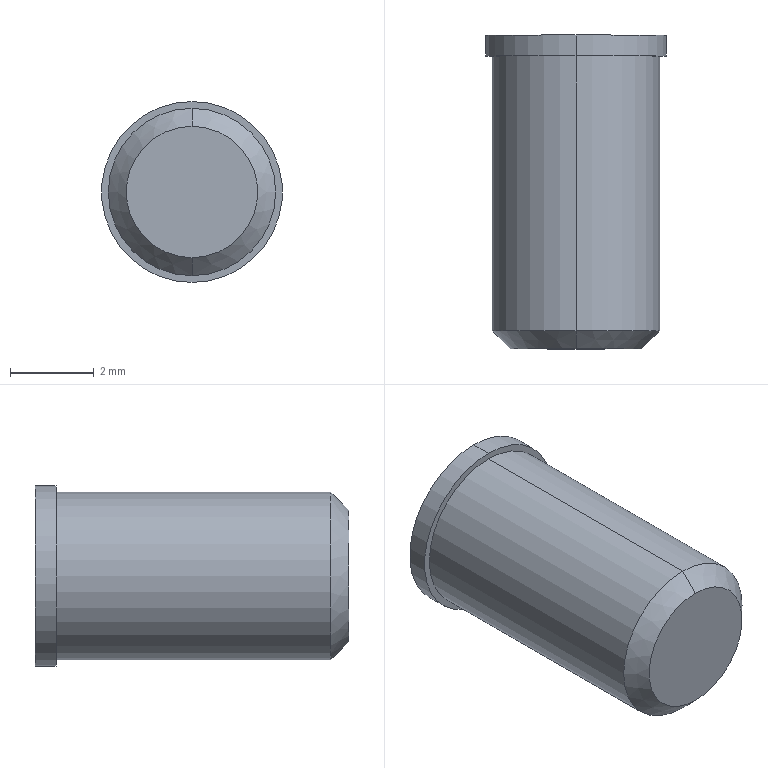Part | STEP file | HG15_PlugScrew | 1 solid | 16 faces | box 4.324 x 7.5 x 4.324 mm | volume 90.944 mm3 | plane 10 | cylinder 4 | cone 2 | commonest cylinder face diameters 4 x2 4.324 x2
STEP:
#1=CARTESIAN_POINT('',(0.,0.,0.));
#2=DIRECTION('',(0.,0.,1.));
#3=DIRECTION('',(1.,0.,0.));
#4=AXIS2_PLACEMENT_3D('',#1,#2,#3);
#5=CARTESIAN_POINT('',(0.,-7.,1.571));
#6=VERTEX_POINT('',#5);
#7=CARTESIAN_POINT('',(0.,-7.,-1.571));
#8=VERTEX_POINT('',#7);
#9=CARTESIAN_POINT('',(0.,-7.,0.));
#10=DIRECTION('',(0.,1.,0.));
#11=DIRECTION('',(0.,0.,1.));
#12=AXIS2_PLACEMENT_3D('',#9,#10,#11);
#13=CIRCLE('',#12,1.571);
#14=CARTESIAN_POINT('',(0.,-7.,0.));
#15=DIRECTION('',(0.,1.,0.));
#16=DIRECTION('',(0.,0.,1.));
#17=AXIS2_PLACEMENT_3D('',#14,#15,#16);
#18=CONICAL_SURFACE('',#17,1.571,0.7854);
#19=CARTESIAN_POINT('',(0.,0.));
#20=DIRECTION('',(1.,0.));
#21=VECTOR('',#20,1.);
#22=LINE('',#19,#21);
#23=(GEOMETRIC_REPRESENTATION_CONTEXT(2)PARAMETRIC_REPRESENTATION_CONTEXT()REPRESENTATION_CONTEXT('',''));
#24=DEFINITIONAL_REPRESENTATION('',(#22),#23);
#25=PCURVE('',#18,#24);
#26=CARTESIAN_POINT('',(1.571,-7.,0.));
#27=DIRECTION('',(0.,1.,0.));
#28=DIRECTION('',(0.,0.,1.));
#29=AXIS2_PLACEMENT_3D('',#26,#27,#28);
#30=PLANE('',#29);
#31=CARTESIAN_POINT('',(0.,-1.571));
#32=DIRECTION('',(1.,0.));
#33=AXIS2_PLACEMENT_2D('',#31,#32);
#34=CIRCLE('',#33,1.571);
#35=(GEOMETRIC_REPRESENTATION_CONTEXT(2)PARAMETRIC_REPRESENTATION_CONTEXT()REPRESENTATION_CONTEXT('',''));
#36=DEFINITIONAL_REPRESENTATION('',(#34),#35);
#37=PCURVE('',#30,#36);
#38=SURFACE_CURVE('',#13,(#25,#37),.PCURVE_S1.);
#39=EDGE_CURVE('',#6,#8,#38,.T.);
#40=ORIENTED_EDGE('',*,*,#39,.T.);
#41=CARTESIAN_POINT('',(0.,-6.571,-2.));
#42=VERTEX_POINT('',#41);
#43=CARTESIAN_POINT('',(0.,-7.,-1.571));
#44=DIRECTION('',(0.,0.7071,-0.7071));
#45=VECTOR('',#44,1.);
#46=LINE('',#43,#45);
#47=CARTESIAN_POINT('',(3.142,0.));
#48=DIRECTION('',(0.,1.));
#49=VECTOR('',#48,1.);
#50=LINE('',#47,#49);
#51=(GEOMETRIC_REPRESENTATION_CONTEXT(2)PARAMETRIC_REPRESENTATION_CONTEXT()REPRESENTATION_CONTEXT('',''));
#52=DEFINITIONAL_REPRESENTATION('',(#50),#51);
#53=PCURVE('',#18,#52);
#54=CARTESIAN_POINT('',(0.,-7.,0.));
#55=DIRECTION('',(0.,1.,0.));
#56=DIRECTION('',(0.,0.,1.));
#57=AXIS2_PLACEMENT_3D('',#54,#55,#56);
#58=CONICAL_SURFACE('',#57,1.571,0.7854);
#59=CARTESIAN_POINT('',(3.142,0.));
#60=DIRECTION('',(0.,1.));
#61=VECTOR('',#60,1.);
#62=LINE('',#59,#61);
#63=(GEOMETRIC_REPRESENTATION_CONTEXT(2)PARAMETRIC_REPRESENTATION_CONTEXT()REPRESENTATION_CONTEXT('',''));
#64=DEFINITIONAL_REPRESENTATION('',(#62),#63);
#65=PCURVE('',#58,#64);
#66=SURFACE_CURVE('',#46,(#53,#65),.PCURVE_S1.);
#67=EDGE_CURVE('',#8,#42,#66,.T.);
#68=ORIENTED_EDGE('',*,*,#67,.T.);
#69=CARTESIAN_POINT('',(0.,-6.571,2.));
#70=VERTEX_POINT('',#69);
#71=CARTESIAN_POINT('',(0.,-6.571,0.));
#72=DIRECTION('',(0.,1.,0.));
#73=DIRECTION('',(0.,0.,1.));
#74=AXIS2_PLACEMENT_3D('',#71,#72,#73);
#75=CIRCLE('',#74,2.);
#76=CARTESIAN_POINT('',(0.,0.4295));
#77=DIRECTION('',(1.,0.));
#78=VECTOR('',#77,1.);
#79=LINE('',#76,#78);
#80=(GEOMETRIC_REPRESENTATION_CONTEXT(2)PARAMETRIC_REPRESENTATION_CONTEXT()REPRESENTATION_CONTEXT('',''));
#81=DEFINITIONAL_REPRESENTATION('',(#79),#80);
#82=PCURVE('',#18,#81);
#83=CARTESIAN_POINT('',(0.,-7.,0.));
#84=DIRECTION('',(0.,1.,0.));
#85=DIRECTION('',(0.,0.,1.));
#86=AXIS2_PLACEMENT_3D('',#83,#84,#85);
#87=CYLINDRICAL_SURFACE('',#86,2.);
#88=CARTESIAN_POINT('',(0.,0.4295));
#89=DIRECTION('',(1.,0.));
#90=VECTOR('',#89,1.);
#91=LINE('',#88,#90);
#92=(GEOMETRIC_REPRESENTATION_CONTEXT(2)PARAMETRIC_REPRESENTATION_CONTEXT()REPRESENTATION_CONTEXT('',''));
#93=DEFINITIONAL_REPRESENTATION('',(#91),#92);
#94=PCURVE('',#87,#93);
#95=SURFACE_CURVE('',#75,(#82,#94),.PCURVE_S1.);
#96=EDGE_CURVE('',#70,#42,#95,.T.);
#97=ORIENTED_EDGE('',*,*,#96,.F.);
#98=CARTESIAN_POINT('',(0.,-7.,1.571));
#99=DIRECTION('',(0.,0.7071,0.7071));
#100=VECTOR('',#99,1.);
#101=LINE('',#98,#100);
#102=CARTESIAN_POINT('',(0.,0.));
#103=DIRECTION('',(0.,1.));
#104=VECTOR('',#103,1.);
#105=LINE('',#102,#104);
#106=(GEOMETRIC_REPRESENTATION_CONTEXT(2)PARAMETRIC_REPRESENTATION_CONTEXT()REPRESENTATION_CONTEXT('',''));
#107=DEFINITIONAL_REPRESENTATION('',(#105),#106);
#108=PCURVE('',#18,#107);
#109=CARTESIAN_POINT('',(6.283,0.));
#110=DIRECTION('',(0.,1.));
#111=VECTOR('',#110,1.);
#112=LINE('',#109,#111);
#113=(GEOMETRIC_REPRESENTATION_CONTEXT(2)PARAMETRIC_REPRESENTATION_CONTEXT()REPRESENTATION_CONTEXT('',''));
#114=DEFINITIONAL_REPRESENTATION('',(#112),#113);
#115=PCURVE('',#58,#114);
#116=SURFACE_CURVE('',#101,(#108,#115),.PCURVE_S1.);
#117=EDGE_CURVE('',#6,#70,#116,.T.);
#118=ORIENTED_EDGE('',*,*,#117,.F.);
#119=EDGE_LOOP('',(#40,#68,#97,#118));
#120=FACE_BOUND('',#119,.T.);
#121=ADVANCED_FACE('',(#120),#18,.T.);
#122=ORIENTED_EDGE('',*,*,#96,.T.);
#123=CARTESIAN_POINT('',(0.,0.,-2.));
#124=VERTEX_POINT('',#123);
#125=CARTESIAN_POINT('',(0.,-7.,-2.));
#126=DIRECTION('',(0.,1.,0.));
#127=VECTOR('',#126,1.);
#128=LINE('',#125,#127);
#129=CARTESIAN_POINT('',(3.142,0.));
#130=DIRECTION('',(0.,1.));
#131=VECTOR('',#130,1.);
#132=LINE('',#129,#131);
#133=(GEOMETRIC_REPRESENTATION_CONTEXT(2)PARAMETRIC_REPRESENTATION_CONTEXT()REPRESENTATION_CONTEXT('',''));
#134=DEFINITIONAL_REPRESENTATION('',(#132),#133);
#135=PCURVE('',#87,#134);
#136=CARTESIAN_POINT('',(0.,-7.,0.));
#137=DIRECTION('',(0.,1.,0.));
#138=DIRECTION('',(0.,0.,1.));
#139=AXIS2_PLACEMENT_3D('',#136,#137,#138);
#140=CYLINDRICAL_SURFACE('',#139,2.);
#141=CARTESIAN_POINT('',(3.142,0.));
#142=DIRECTION('',(0.,1.));
#143=VECTOR('',#142,1.);
#144=LINE('',#141,#143);
#145=(GEOMETRIC_REPRESENTATION_CONTEXT(2)PARAMETRIC_REPRESENTATION_CONTEXT()REPRESENTATION_CONTEXT('',''));
#146=DEFINITIONAL_REPRESENTATION('',(#144),#145);
#147=PCURVE('',#140,#146);
#148=SURFACE_CURVE('',#128,(#135,#147),.PCURVE_S1.);
#149=EDGE_CURVE('',#42,#124,#148,.T.);
#150=ORIENTED_EDGE('',*,*,#149,.T.);
#151=CARTESIAN_POINT('',(0.,0.,2.));
#152=VERTEX_POINT('',#151);
#153=CARTESIAN_POINT('',(0.,0.,0.));
#154=DIRECTION('',(0.,1.,0.));
#155=DIRECTION('',(0.,0.,1.));
#156=AXIS2_PLACEMENT_3D('',#153,#154,#155);
#157=CIRCLE('',#156,2.);
#158=CARTESIAN_POINT('',(0.,7.));
#159=DIRECTION('',(1.,0.));
#160=VECTOR('',#159,1.);
#161=LINE('',#158,#160);
#162=(GEOMETRIC_REPRESENTATION_CONTEXT(2)PARAMETRIC_REPRESENTATION_CONTEXT()REPRESENTATION_CONTEXT('',''));
#163=DEFINITIONAL_REPRESENTATION('',(#161),#162);
#164=PCURVE('',#87,#163);
#165=CARTESIAN_POINT('',(2.162,0.,0.));
#166=DIRECTION('',(0.,1.,0.));
#167=DIRECTION('',(0.,0.,1.));
#168=AXIS2_PLACEMENT_3D('',#165,#166,#167);
#169=PLANE('',#168);
#170=CARTESIAN_POINT('',(0.,-2.162));
#171=DIRECTION('',(1.,0.));
#172=AXIS2_PLACEMENT_2D('',#170,#171);
#173=CIRCLE('',#172,2.);
#174=(GEOMETRIC_REPRESENTATION_CONTEXT(2)PARAMETRIC_REPRESENTATION_CONTEXT()REPRESENTATION_CONTEXT('',''));
#175=DEFINITIONAL_REPRESENTATION('',(#173),#174);
#176=PCURVE('',#169,#175);
#177=SURFACE_CURVE('',#157,(#164,#176),.PCURVE_S1.);
#178=EDGE_CURVE('',#152,#124,#177,.T.);
#179=ORIENTED_EDGE('',*,*,#178,.F.);
#180=CARTESIAN_POINT('',(0.,-7.,2.));
#181=DIRECTION('',(0.,1.,0.));
#182=VECTOR('',#181,1.);
#183=LINE('',#180,#182);
#184=CARTESIAN_POINT('',(0.,0.));
#185=DIRECTION('',(0.,1.));
#186=VECTOR('',#185,1.);
#187=LINE('',#184,#186);
#188=(GEOMETRIC_REPRESENTATION_CONTEXT(2)PARAMETRIC_REPRESENTATION_CONTEXT()REPRESENTATION_CONTEXT('',''));
#189=DEFINITIONAL_REPRESENTATION('',(#187),#188);
#190=PCURVE('',#87,#189);
#191=CARTESIAN_POINT('',(6.283,0.));
#192=DIRECTION('',(0.,1.));
#193=VECTOR('',#192,1.);
#194=LINE('',#191,#193);
#195=(GEOMETRIC_REPRESENTATION_CONTEXT(2)PARAMETRIC_REPRESENTATION_CONTEXT()REPRESENTATION_CONTEXT('',''));
#196=DEFINITIONAL_REPRESENTATION('',(#194),#195);
#197=PCURVE('',#140,#196);
#198=SURFACE_CURVE('',#183,(#190,#197),.PCURVE_S1.);
#199=EDGE_CURVE('',#70,#152,#198,.T.);
#200=ORIENTED_EDGE('',*,*,#199,.F.);
#201=EDGE_LOOP('',(#122,#150,#179,#200));
#202=FACE_BOUND('',#201,.T.);
#203=ADVANCED_FACE('',(#202),#87,.T.);
#204=CARTESIAN_POINT('',(0.,0.,2.162));
#205=VERTEX_POINT('',#204);
#206=CARTESIAN_POINT('',(0.,0.,-2.162));
#207=VERTEX_POINT('',#206);
#208=CARTESIAN_POINT('',(0.,0.,0.));
#209=DIRECTION('',(0.,1.,0.));
#210=DIRECTION('',(0.,0.,1.));
#211=AXIS2_PLACEMENT_3D('',#208,#209,#210);
#212=CIRCLE('',#211,2.162);
#213=CARTESIAN_POINT('',(0.,-7.,0.));
#214=DIRECTION('',(0.,1.,0.));
#215=DIRECTION('',(0.,0.,1.));
#216=AXIS2_PLACEMENT_3D('',#213,#214,#215);
#217=CYLINDRICAL_SURFACE('',#216,2.162);
#218=CARTESIAN_POINT('',(0.,7.));
#219=DIRECTION('',(1.,0.));
#220=VECTOR('',#219,1.);
#221=LINE('',#218,#220);
#222=(GEOMETRIC_REPRESENTATION_CONTEXT(2)PARAMETRIC_REPRESENTATION_CONTEXT()REPRESENTATION_CONTEXT('',''));
#223=DEFINITIONAL_REPRESENTATION('',(#221),#222);
#224=PCURVE('',#217,#223);
#225=CARTESIAN_POINT('',(0.,-2.162));
#226=DIRECTION('',(1.,0.));
#227=AXIS2_PLACEMENT_2D('',#225,#226);
#228=CIRCLE('',#227,2.162);
#229=(GEOMETRIC_REPRESENTATION_CONTEXT(2)PARAMETRIC_REPRESENTATION_CONTEXT()REPRESENTATION_CONTEXT('',''));
#230=DEFINITIONAL_REPRESENTATION('',(#228),#229);
#231=PCURVE('',#169,#230);
#232=SURFACE_CURVE('',#212,(#224,#231),.PCURVE_S1.);
#233=EDGE_CURVE('',#205,#207,#232,.T.);
#234=ORIENTED_EDGE('',*,*,#233,.T.);
#235=CARTESIAN_POINT('',(0.,0.5,-2.162));
#236=VERTEX_POINT('',#235);
#237=CARTESIAN_POINT('',(0.,-7.,-2.162));
#238=DIRECTION('',(0.,1.,0.));
#239=VECTOR('',#238,1.);
#240=LINE('',#237,#239);
#241=CARTESIAN_POINT('',(3.142,0.));
#242=DIRECTION('',(0.,1.));
#243=VECTOR('',#242,1.);
#244=LINE('',#241,#243);
#245=(GEOMETRIC_REPRESENTATION_CONTEXT(2)PARAMETRIC_REPRESENTATION_CONTEXT()REPRESENTATION_CONTEXT('',''));
#246=DEFINITIONAL_REPRESENTATION('',(#244),#245);
#247=PCURVE('',#217,#246);
#248=CARTESIAN_POINT('',(0.,-7.,0.));
#249=DIRECTION('',(0.,1.,0.));
#250=DIRECTION('',(0.,0.,1.));
#251=AXIS2_PLACEMENT_3D('',#248,#249,#250);
#252=CYLINDRICAL_SURFACE('',#251,2.162);
#253=CARTESIAN_POINT('',(3.142,0.));
#254=DIRECTION('',(0.,1.));
#255=VECTOR('',#254,1.);
#256=LINE('',#253,#255);
#257=(GEOMETRIC_REPRESENTATION_CONTEXT(2)PARAMETRIC_REPRESENTATION_CONTEXT()REPRESENTATION_CONTEXT('',''));
#258=DEFINITIONAL_REPRESENTATION('',(#256),#257);
#259=PCURVE('',#252,#258);
#260=SURFACE_CURVE('',#240,(#247,#259),.PCURVE_S1.);
#261=EDGE_CURVE('',#207,#236,#260,.T.);
#262=ORIENTED_EDGE('',*,*,#261,.T.);
#263=CARTESIAN_POINT('',(0.,0.5,2.162));
#264=VERTEX_POINT('',#263);
#265=CARTESIAN_POINT('',(0.,0.5,0.));
#266=DIRECTION('',(0.,1.,0.));
#267=DIRECTION('',(0.,0.,1.));
#268=AXIS2_PLACEMENT_3D('',#265,#266,#267);
#269=CIRCLE('',#268,2.162);
#270=CARTESIAN_POINT('',(0.,7.5));
#271=DIRECTION('',(1.,0.));
#272=VECTOR('',#271,1.);
#273=LINE('',#270,#272);
#274=(GEOMETRIC_REPRESENTATION_CONTEXT(2)PARAMETRIC_REPRESENTATION_CONTEXT()REPRESENTATION_CONTEXT('',''));
#275=DEFINITIONAL_REPRESENTATION('',(#273),#274);
#276=PCURVE('',#217,#275);
#277=CARTESIAN_POINT('',(0.,0.5,0.));
#278=DIRECTION('',(0.,-1.,0.));
#279=DIRECTION('',(0.,0.,-1.));
#280=AXIS2_PLACEMENT_3D('',#277,#278,#279);
#281=PLANE('',#280);
#282=CARTESIAN_POINT('',(-2.162,0.));
#283=CARTESIAN_POINT('',(-2.162,3.745));
#284=CARTESIAN_POINT('',(1.081,1.872));
#285=CARTESIAN_POINT('',(4.324,0.));
#286=CARTESIAN_POINT('',(1.081,-1.872));
#287=CARTESIAN_POINT('',(-2.162,-3.745));
#288=CARTESIAN_POINT('',(-2.162,0.));
#289=(BOUNDED_CURVE()B_SPLINE_CURVE(2,(#282,#283,#284,#285,#286,#287,#288),.UNSPECIFIED.,.T.,.F.)B_SPLINE_CURVE_WITH_KNOTS((1,2,2,2,2,1),(-2.094,0.,2.094,4.189,6.283,8.378),.UNSPECIFIED.)CURVE()GEOMETRIC_REPRESENTATION_ITEM()RATIONAL_B_SPLINE_CURVE((1.,0.5,1.,0.5,1.,0.5,1.))REPRESENTATION_ITEM(''));
#290=(GEOMETRIC_REPRESENTATION_CONTEXT(2)PARAMETRIC_REPRESENTATION_CONTEXT()REPRESENTATION_CONTEXT('',''));
#291=DEFINITIONAL_REPRESENTATION('',(#289),#290);
#292=PCURVE('',#281,#291);
#293=SURFACE_CURVE('',#269,(#276,#292),.PCURVE_S1.);
#294=EDGE_CURVE('',#264,#236,#293,.T.);
#295=ORIENTED_EDGE('',*,*,#294,.F.);
#296=CARTESIAN_POINT('',(0.,-7.,2.162));
#297=DIRECTION('',(0.,1.,0.));
#298=VECTOR('',#297,1.);
#299=LINE('',#296,#298);
#300=CARTESIAN_POINT('',(0.,0.));
#301=DIRECTION('',(0.,1.));
#302=VECTOR('',#301,1.);
#303=LINE('',#300,#302);
#304=(GEOMETRIC_REPRESENTATION_CONTEXT(2)PARAMETRIC_REPRESENTATION_CONTEXT()REPRESENTATION_CONTEXT('',''));
#305=DEFINITIONAL_REPRESENTATION('',(#303),#304);
#306=PCURVE('',#217,#305);
#307=CARTESIAN_POINT('',(6.283,0.));
#308=DIRECTION('',(0.,1.));
#309=VECTOR('',#308,1.);
#310=LINE('',#307,#309);
#311=(GEOMETRIC_REPRESENTATION_CONTEXT(2)PARAMETRIC_REPRESENTATION_CONTEXT()REPRESENTATION_CONTEXT('',''));
#312=DEFINITIONAL_REPRESENTATION('',(#310),#311);
#313=PCURVE('',#252,#312);
#314=SURFACE_CURVE('',#299,(#306,#313),.PCURVE_S1.);
#315=EDGE_CURVE('',#205,#264,#314,.T.);
#316=ORIENTED_EDGE('',*,*,#315,.F.);
#317=EDGE_LOOP('',(#234,#262,#295,#316));
#318=FACE_BOUND('',#317,.T.);
#319=ADVANCED_FACE('',(#318),#217,.T.);
#320=CARTESIAN_POINT('',(-1.125,0.5,0.6495));
#321=VERTEX_POINT('',#320);
#322=CARTESIAN_POINT('',(0.,0.5,1.299));
#323=VERTEX_POINT('',#322);
#324=CARTESIAN_POINT('',(-1.125,0.5,0.6495));
#325=DIRECTION('',(0.866,0.,0.5));
#326=VECTOR('',#325,1.);
#327=LINE('',#324,#326);
#328=CARTESIAN_POINT('',(-0.6495,-1.125));
#329=DIRECTION('',(-0.5,0.866));
#330=VECTOR('',#329,1.);
#331=LINE('',#328,#330);
#332=(GEOMETRIC_REPRESENTATION_CONTEXT(2)PARAMETRIC_REPRESENTATION_CONTEXT()REPRESENTATION_CONTEXT('',''));
#333=DEFINITIONAL_REPRESENTATION('',(#331),#332);
#334=PCURVE('',#281,#333);
#335=CARTESIAN_POINT('',(-1.125,-0.25,0.6495));
#336=DIRECTION('',(-0.5,0.,0.866));
#337=DIRECTION('',(0.866,0.,0.5));
#338=AXIS2_PLACEMENT_3D('',#335,#336,#337);
#339=PLANE('',#338);
#340=CARTESIAN_POINT('',(0.,0.75));
#341=DIRECTION('',(1.,0.));
#342=VECTOR('',#341,1.);
#343=LINE('',#340,#342);
#344=(GEOMETRIC_REPRESENTATION_CONTEXT(2)PARAMETRIC_REPRESENTATION_CONTEXT()REPRESENTATION_CONTEXT('',''));
#345=DEFINITIONAL_REPRESENTATION('',(#343),#344);
#346=PCURVE('',#339,#345);
#347=SURFACE_CURVE('',#327,(#334,#346),.PCURVE_S1.);
#348=EDGE_CURVE('',#321,#323,#347,.T.);
#349=ORIENTED_EDGE('',*,*,#348,.F.);
#350=CARTESIAN_POINT('',(-1.125,0.5,-0.6495));
#351=VERTEX_POINT('',#350);
#352=CARTESIAN_POINT('',(-1.125,0.5,-0.6495));
#353=DIRECTION('',(0.,0.,1.));
#354=VECTOR('',#353,1.);
#355=LINE('',#352,#354);
#356=CARTESIAN_POINT('',(0.6495,-1.125));
#357=DIRECTION('',(-1.,0.));
#358=VECTOR('',#357,1.);
#359=LINE('',#356,#358);
#360=(GEOMETRIC_REPRESENTATION_CONTEXT(2)PARAMETRIC_REPRESENTATION_CONTEXT()REPRESENTATION_CONTEXT('',''));
#361=DEFINITIONAL_REPRESENTATION('',(#359),#360);
#362=PCURVE('',#281,#361);
#363=CARTESIAN_POINT('',(-1.125,-0.25,-0.6495));
#364=DIRECTION('',(-1.,0.,0.));
#365=DIRECTION('',(0.,0.,1.));
#366=AXIS2_PLACEMENT_3D('',#363,#364,#365);
#367=PLANE('',#366);
#368=CARTESIAN_POINT('',(0.,0.75));
#369=DIRECTION('',(1.,0.));
#370=VECTOR('',#369,1.);
#371=LINE('',#368,#370);
#372=(GEOMETRIC_REPRESENTATION_CONTEXT(2)PARAMETRIC_REPRESENTATION_CONTEXT()REPRESENTATION_CONTEXT('',''));
#373=DEFINITIONAL_REPRESENTATION('',(#371),#372);
#374=PCURVE('',#367,#373);
#375=SURFACE_CURVE('',#355,(#362,#374),.PCURVE_S1.);
#376=EDGE_CURVE('',#351,#321,#375,.T.);
#377=ORIENTED_EDGE('',*,*,#376,.F.);
#378=CARTESIAN_POINT('',(0.,0.5,-1.299));
#379=VERTEX_POINT('',#378);
#380=CARTESIAN_POINT('',(0.,0.5,-1.299));
#381=DIRECTION('',(-0.866,0.,0.5));
#382=VECTOR('',#381,1.);
#383=LINE('',#380,#382);
#384=CARTESIAN_POINT('',(1.299,0.));
#385=DIRECTION('',(-0.5,-0.866));
#386=VECTOR('',#385,1.);
#387=LINE('',#384,#386);
#388=(GEOMETRIC_REPRESENTATION_CONTEXT(2)PARAMETRIC_REPRESENTATION_CONTEXT()REPRESENTATION_CONTEXT('',''));
#389=DEFINITIONAL_REPRESENTATION('',(#387),#388);
#390=PCURVE('',#281,#389);
#391=CARTESIAN_POINT('',(0.,-0.25,-1.299));
#392=DIRECTION('',(-0.5,0.,-0.866));
#393=DIRECTION('',(-0.866,0.,0.5));
#394=AXIS2_PLACEMENT_3D('',#391,#392,#393);
#395=PLANE('',#394);
#396=CARTESIAN_POINT('',(0.,0.75));
#397=DIRECTION('',(1.,0.));
#398=VECTOR('',#397,1.);
#399=LINE('',#396,#398);
#400=(GEOMETRIC_REPRESENTATION_CONTEXT(2)PARAMETRIC_REPRESENTATION_CONTEXT()REPRESENTATION_CONTEXT('',''));
#401=DEFINITIONAL_REPRESENTATION('',(#399),#400);
#402=PCURVE('',#395,#401);
#403=SURFACE_CURVE('',#383,(#390,#402),.PCURVE_S1.);
#404=EDGE_CURVE('',#379,#351,#403,.T.);
#405=ORIENTED_EDGE('',*,*,#404,.F.);
#406=CARTESIAN_POINT('',(1.125,0.5,-0.6495));
#407=VERTEX_POINT('',#406);
#408=CARTESIAN_POINT('',(1.125,0.5,-0.6495));
#409=DIRECTION('',(-0.866,0.,-0.5));
#410=VECTOR('',#409,1.);
#411=LINE('',#408,#410);
#412=CARTESIAN_POINT('',(0.6495,1.125));
#413=DIRECTION('',(0.5,-0.866));
#414=VECTOR('',#413,1.);
#415=LINE('',#412,#414);
#416=(GEOMETRIC_REPRESENTATION_CONTEXT(2)PARAMETRIC_REPRESENTATION_CONTEXT()REPRESENTATION_CONTEXT('',''));
#417=DEFINITIONAL_REPRESENTATION('',(#415),#416);
#418=PCURVE('',#281,#417);
#419=CARTESIAN_POINT('',(1.125,-0.25,-0.6495));
#420=DIRECTION('',(0.5,0.,-0.866));
#421=DIRECTION('',(-0.866,0.,-0.5));
#422=AXIS2_PLACEMENT_3D('',#419,#420,#421);
#423=PLANE('',#422);
#424=CARTESIAN_POINT('',(0.,0.75));
#425=DIRECTION('',(1.,0.));
#426=VECTOR('',#425,1.);
#427=LINE('',#424,#426);
#428=(GEOMETRIC_REPRESENTATION_CONTEXT(2)PARAMETRIC_REPRESENTATION_CONTEXT()REPRESENTATION_CONTEXT('',''));
#429=DEFINITIONAL_REPRESENTATION('',(#427),#428);
#430=PCURVE('',#423,#429);
#431=SURFACE_CURVE('',#411,(#418,#430),.PCURVE_S1.);
#432=EDGE_CURVE('',#407,#379,#431,.T.);
#433=ORIENTED_EDGE('',*,*,#432,.F.);
#434=CARTESIAN_POINT('',(1.125,0.5,0.6495));
#435=VERTEX_POINT('',#434);
#436=CARTESIAN_POINT('',(1.125,0.5,0.6495));
#437=DIRECTION('',(0.,0.,-1.));
#438=VECTOR('',#437,1.);
#439=LINE('',#436,#438);
#440=CARTESIAN_POINT('',(-0.6495,1.125));
#441=DIRECTION('',(1.,0.));
#442=VECTOR('',#441,1.);
#443=LINE('',#440,#442);
#444=(GEOMETRIC_REPRESENTATION_CONTEXT(2)PARAMETRIC_REPRESENTATION_CONTEXT()REPRESENTATION_CONTEXT('',''));
#445=DEFINITIONAL_REPRESENTATION('',(#443),#444);
#446=PCURVE('',#281,#445);
#447=CARTESIAN_POINT('',(1.125,-0.25,0.6495));
#448=DIRECTION('',(1.,0.,0.));
#449=DIRECTION('',(0.,0.,-1.));
#450=AXIS2_PLACEMENT_3D('',#447,#448,#449);
#451=PLANE('',#450);
#452=CARTESIAN_POINT('',(0.,0.75));
#453=DIRECTION('',(1.,0.));
#454=VECTOR('',#453,1.);
#455=LINE('',#452,#454);
#456=(GEOMETRIC_REPRESENTATION_CONTEXT(2)PARAMETRIC_REPRESENTATION_CONTEXT()REPRESENTATION_CONTEXT('',''));
#457=DEFINITIONAL_REPRESENTATION('',(#455),#456);
#458=PCURVE('',#451,#457);
#459=SURFACE_CURVE('',#439,(#446,#458),.PCURVE_S1.);
#460=EDGE_CURVE('',#435,#407,#459,.T.);
#461=ORIENTED_EDGE('',*,*,#460,.F.);
#462=CARTESIAN_POINT('',(0.,0.5,1.299));
#463=DIRECTION('',(0.866,0.,-0.5));
#464=VECTOR('',#463,1.);
#465=LINE('',#462,#464);
#466=CARTESIAN_POINT('',(-1.299,0.));
#467=DIRECTION('',(0.5,0.866));
#468=VECTOR('',#467,1.);
#469=LINE('',#466,#468);
#470=(GEOMETRIC_REPRESENTATION_CONTEXT(2)PARAMETRIC_REPRESENTATION_CONTEXT()REPRESENTATION_CONTEXT('',''));
#471=DEFINITIONAL_REPRESENTATION('',(#469),#470);
#472=PCURVE('',#281,#471);
#473=CARTESIAN_POINT('',(0.,-0.25,1.299));
#474=DIRECTION('',(0.5,0.,0.866));
#475=DIRECTION('',(0.866,0.,-0.5));
#476=AXIS2_PLACEMENT_3D('',#473,#474,#475);
#477=PLANE('',#476);
#478=CARTESIAN_POINT('',(0.,0.75));
#479=DIRECTION('',(1.,0.));
#480=VECTOR('',#479,1.);
#481=LINE('',#478,#480);
#482=(GEOMETRIC_REPRESENTATION_CONTEXT(2)PARAMETRIC_REPRESENTATION_CONTEXT()REPRESENTATION_CONTEXT('',''));
#483=DEFINITIONAL_REPRESENTATION('',(#481),#482);
#484=PCURVE('',#477,#483);
#485=SURFACE_CURVE('',#465,(#472,#484),.PCURVE_S1.);
#486=EDGE_CURVE('',#323,#435,#485,.T.);
#487=ORIENTED_EDGE('',*,*,#486,.F.);
#488=EDGE_LOOP('',(#349,#377,#405,#433,#461,#487));
#489=FACE_BOUND('',#488,.T.);
#490=ORIENTED_EDGE('',*,*,#294,.T.);
#491=CARTESIAN_POINT('',(0.,0.5,0.));
#492=DIRECTION('',(0.,1.,0.));
#493=DIRECTION('',(0.,0.,1.));
#494=AXIS2_PLACEMENT_3D('',#491,#492,#493);
#495=CIRCLE('',#494,2.162);
#496=CARTESIAN_POINT('',(-2.162,0.));
#497=CARTESIAN_POINT('',(-2.162,3.745));
#498=CARTESIAN_POINT('',(1.081,1.872));
#499=CARTESIAN_POINT('',(4.324,0.));
#500=CARTESIAN_POINT('',(1.081,-1.872));
#501=CARTESIAN_POINT('',(-2.162,-3.745));
#502=CARTESIAN_POINT('',(-2.162,0.));
#503=(BOUNDED_CURVE()B_SPLINE_CURVE(2,(#496,#497,#498,#499,#500,#501,#502),.UNSPECIFIED.,.T.,.F.)B_SPLINE_CURVE_WITH_KNOTS((1,2,2,2,2,1),(-2.094,0.,2.094,4.189,6.283,8.378),.UNSPECIFIED.)CURVE()GEOMETRIC_REPRESENTATION_ITEM()RATIONAL_B_SPLINE_CURVE((1.,0.5,1.,0.5,1.,0.5,1.))REPRESENTATION_ITEM(''));
#504=(GEOMETRIC_REPRESENTATION_CONTEXT(2)PARAMETRIC_REPRESENTATION_CONTEXT()REPRESENTATION_CONTEXT('',''));
#505=DEFINITIONAL_REPRESENTATION('',(#503),#504);
#506=PCURVE('',#281,#505);
#507=CARTESIAN_POINT('',(0.,7.5));
#508=DIRECTION('',(1.,0.));
#509=VECTOR('',#508,1.);
#510=LINE('',#507,#509);
#511=(GEOMETRIC_REPRESENTATION_CONTEXT(2)PARAMETRIC_REPRESENTATION_CONTEXT()REPRESENTATION_CONTEXT('',''));
#512=DEFINITIONAL_REPRESENTATION('',(#510),#511);
#513=PCURVE('',#252,#512);
#514=SURFACE_CURVE('',#495,(#506,#513),.PCURVE_S1.);
#515=EDGE_CURVE('',#236,#264,#514,.T.);
#516=ORIENTED_EDGE('',*,*,#515,.T.);
#517=EDGE_LOOP('',(#490,#516));
#518=FACE_BOUND('',#517,.T.);
#519=ADVANCED_FACE('',(#489,#518),#281,.F.);
#520=ORIENTED_EDGE('',*,*,#261,.F.);
#521=CARTESIAN_POINT('',(0.,0.,0.));
#522=DIRECTION('',(0.,1.,0.));
#523=DIRECTION('',(0.,0.,1.));
#524=AXIS2_PLACEMENT_3D('',#521,#522,#523);
#525=CIRCLE('',#524,2.162);
#526=CARTESIAN_POINT('',(0.,7.));
#527=DIRECTION('',(1.,0.));
#528=VECTOR('',#527,1.);
#529=LINE('',#526,#528);
#530=(GEOMETRIC_REPRESENTATION_CONTEXT(2)PARAMETRIC_REPRESENTATION_CONTEXT()REPRESENTATION_CONTEXT('',''));
#531=DEFINITIONAL_REPRESENTATION('',(#529),#530);
#532=PCURVE('',#252,#531);
#533=CARTESIAN_POINT('',(0.,-2.162));
#534=DIRECTION('',(1.,0.));
#535=AXIS2_PLACEMENT_2D('',#533,#534);
#536=CIRCLE('',#535,2.162);
#537=(GEOMETRIC_REPRESENTATION_CONTEXT(2)PARAMETRIC_REPRESENTATION_CONTEXT()REPRESENTATION_CONTEXT('',''));
#538=DEFINITIONAL_REPRESENTATION('',(#536),#537);
#539=PCURVE('',#169,#538);
#540=SURFACE_CURVE('',#525,(#532,#539),.PCURVE_S1.);
#541=EDGE_CURVE('',#207,#205,#540,.T.);
#542=ORIENTED_EDGE('',*,*,#541,.T.);
#543=ORIENTED_EDGE('',*,*,#315,.T.);
#544=ORIENTED_EDGE('',*,*,#515,.F.);
#545=EDGE_LOOP('',(#520,#542,#543,#544));
#546=FACE_BOUND('',#545,.T.);
#547=ADVANCED_FACE('',(#546),#252,.T.);
#548=ORIENTED_EDGE('',*,*,#233,.F.);
#549=ORIENTED_EDGE('',*,*,#541,.F.);
#550=EDGE_LOOP('',(#548,#549));
#551=FACE_BOUND('',#550,.T.);
#552=ORIENTED_EDGE('',*,*,#178,.T.);
#553=CARTESIAN_POINT('',(0.,0.,0.));
#554=DIRECTION('',(0.,1.,0.));
#555=DIRECTION('',(0.,0.,1.));
#556=AXIS2_PLACEMENT_3D('',#553,#554,#555);
#557=CIRCLE('',#556,2.);
#558=CARTESIAN_POINT('',(0.,-2.162));
#559=DIRECTION('',(1.,0.));
#560=AXIS2_PLACEMENT_2D('',#558,#559);
#561=CIRCLE('',#560,2.);
#562=(GEOMETRIC_REPRESENTATION_CONTEXT(2)PARAMETRIC_REPRESENTATION_CONTEXT()REPRESENTATION_CONTEXT('',''));
#563=DEFINITIONAL_REPRESENTATION('',(#561),#562);
#564=PCURVE('',#169,#563);
#565=CARTESIAN_POINT('',(0.,7.));
#566=DIRECTION('',(1.,0.));
#567=VECTOR('',#566,1.);
#568=LINE('',#565,#567);
#569=(GEOMETRIC_REPRESENTATION_CONTEXT(2)PARAMETRIC_REPRESENTATION_CONTEXT()REPRESENTATION_CONTEXT('',''));
#570=DEFINITIONAL_REPRESENTATION('',(#568),#569);
#571=PCURVE('',#140,#570);
#572=SURFACE_CURVE('',#557,(#564,#571),.PCURVE_S1.);
#573=EDGE_CURVE('',#124,#152,#572,.T.);
#574=ORIENTED_EDGE('',*,*,#573,.T.);
#575=EDGE_LOOP('',(#552,#574));
#576=FACE_BOUND('',#575,.T.);
#577=ADVANCED_FACE('',(#551,#576),#169,.F.);
#578=ORIENTED_EDGE('',*,*,#149,.F.);
#579=CARTESIAN_POINT('',(0.,-6.571,0.));
#580=DIRECTION('',(0.,1.,0.));
#581=DIRECTION('',(0.,0.,1.));
#582=AXIS2_PLACEMENT_3D('',#579,#580,#581);
#583=CIRCLE('',#582,2.);
#584=CARTESIAN_POINT('',(0.,0.4295));
#585=DIRECTION('',(1.,0.));
#586=VECTOR('',#585,1.);
#587=LINE('',#584,#586);
#588=(GEOMETRIC_REPRESENTATION_CONTEXT(2)PARAMETRIC_REPRESENTATION_CONTEXT()REPRESENTATION_CONTEXT('',''));
#589=DEFINITIONAL_REPRESENTATION('',(#587),#588);
#590=PCURVE('',#140,#589);
#591=CARTESIAN_POINT('',(0.,0.4295));
#592=DIRECTION('',(1.,0.));
#593=VECTOR('',#592,1.);
#594=LINE('',#591,#593);
#595=(GEOMETRIC_REPRESENTATION_CONTEXT(2)PARAMETRIC_REPRESENTATION_CONTEXT()REPRESENTATION_CONTEXT('',''));
#596=DEFINITIONAL_REPRESENTATION('',(#594),#595);
#597=PCURVE('',#58,#596);
#598=SURFACE_CURVE('',#583,(#590,#597),.PCURVE_S1.);
#599=EDGE_CURVE('',#42,#70,#598,.T.);
#600=ORIENTED_EDGE('',*,*,#599,.T.);
#601=ORIENTED_EDGE('',*,*,#199,.T.);
#602=ORIENTED_EDGE('',*,*,#573,.F.);
#603=EDGE_LOOP('',(#578,#600,#601,#602));
#604=FACE_BOUND('',#603,.T.);
#605=ADVANCED_FACE('',(#604),#140,.T.);
#606=ORIENTED_EDGE('',*,*,#67,.F.);
#607=CARTESIAN_POINT('',(0.,-7.,0.));
#608=DIRECTION('',(0.,1.,0.));
#609=DIRECTION('',(0.,0.,1.));
#610=AXIS2_PLACEMENT_3D('',#607,#608,#609);
#611=CIRCLE('',#610,1.571);
#612=CARTESIAN_POINT('',(0.,0.));
#613=DIRECTION('',(1.,0.));
#614=VECTOR('',#613,1.);
#615=LINE('',#612,#614);
#616=(GEOMETRIC_REPRESENTATION_CONTEXT(2)PARAMETRIC_REPRESENTATION_CONTEXT()REPRESENTATION_CONTEXT('',''));
#617=DEFINITIONAL_REPRESENTATION('',(#615),#616);
#618=PCURVE('',#58,#617);
#619=CARTESIAN_POINT('',(0.,-1.571));
#620=DIRECTION('',(1.,0.));
#621=AXIS2_PLACEMENT_2D('',#619,#620);
#622=CIRCLE('',#621,1.571);
#623=(GEOMETRIC_REPRESENTATION_CONTEXT(2)PARAMETRIC_REPRESENTATION_CONTEXT()REPRESENTATION_CONTEXT('',''));
#624=DEFINITIONAL_REPRESENTATION('',(#622),#623);
#625=PCURVE('',#30,#624);
#626=SURFACE_CURVE('',#611,(#618,#625),.PCURVE_S1.);
#627=EDGE_CURVE('',#8,#6,#626,.T.);
#628=ORIENTED_EDGE('',*,*,#627,.T.);
#629=ORIENTED_EDGE('',*,*,#117,.T.);
#630=ORIENTED_EDGE('',*,*,#599,.F.);
#631=EDGE_LOOP('',(#606,#628,#629,#630));
#632=FACE_BOUND('',#631,.T.);
#633=ADVANCED_FACE('',(#632),#58,.T.);
#634=ORIENTED_EDGE('',*,*,#39,.F.);
#635=ORIENTED_EDGE('',*,*,#627,.F.);
#636=EDGE_LOOP('',(#634,#635));
#637=FACE_BOUND('',#636,.T.);
#638=ADVANCED_FACE('',(#637),#30,.F.);
#639=ORIENTED_EDGE('',*,*,#376,.T.);
#640=CARTESIAN_POINT('',(-1.125,-0.25,0.6495));
#641=VERTEX_POINT('',#640);
#642=CARTESIAN_POINT('',(-1.125,-0.25,0.6495));
#643=DIRECTION('',(0.,1.,0.));
#644=VECTOR('',#643,1.);
#645=LINE('',#642,#644);
#646=CARTESIAN_POINT('',(1.299,0.));
#647=DIRECTION('',(0.,1.));
#648=VECTOR('',#647,1.);
#649=LINE('',#646,#648);
#650=(GEOMETRIC_REPRESENTATION_CONTEXT(2)PARAMETRIC_REPRESENTATION_CONTEXT()REPRESENTATION_CONTEXT('',''));
#651=DEFINITIONAL_REPRESENTATION('',(#649),#650);
#652=PCURVE('',#367,#651);
#653=CARTESIAN_POINT('',(0.,0.));
#654=DIRECTION('',(0.,1.));
#655=VECTOR('',#654,1.);
#656=LINE('',#653,#655);
#657=(GEOMETRIC_REPRESENTATION_CONTEXT(2)PARAMETRIC_REPRESENTATION_CONTEXT()REPRESENTATION_CONTEXT('',''));
#658=DEFINITIONAL_REPRESENTATION('',(#656),#657);
#659=PCURVE('',#339,#658);
#660=SURFACE_CURVE('',#645,(#652,#659),.PCURVE_S1.);
#661=EDGE_CURVE('',#641,#321,#660,.T.);
#662=ORIENTED_EDGE('',*,*,#661,.F.);
#663=CARTESIAN_POINT('',(-1.125,-0.25,-0.6495));
#664=VERTEX_POINT('',#663);
#665=CARTESIAN_POINT('',(-1.125,-0.25,-0.6495));
#666=DIRECTION('',(0.,0.,1.));
#667=VECTOR('',#666,1.);
#668=LINE('',#665,#667);
#669=CARTESIAN_POINT('',(0.,0.));
#670=DIRECTION('',(1.,0.));
#671=VECTOR('',#670,1.);
#672=LINE('',#669,#671);
#673=(GEOMETRIC_REPRESENTATION_CONTEXT(2)PARAMETRIC_REPRESENTATION_CONTEXT()REPRESENTATION_CONTEXT('',''));
#674=DEFINITIONAL_REPRESENTATION('',(#672),#673);
#675=PCURVE('',#367,#674);
#676=CARTESIAN_POINT('',(0.,-0.25,0.));
#677=DIRECTION('',(0.,1.,0.));
#678=DIRECTION('',(0.,0.,1.));
#679=AXIS2_PLACEMENT_3D('',#676,#677,#678);
#680=PLANE('',#679);
#681=CARTESIAN_POINT('',(-0.6495,-1.125));
#682=DIRECTION('',(1.,0.));
#683=VECTOR('',#682,1.);
#684=LINE('',#681,#683);
#685=(GEOMETRIC_REPRESENTATION_CONTEXT(2)PARAMETRIC_REPRESENTATION_CONTEXT()REPRESENTATION_CONTEXT('',''));
#686=DEFINITIONAL_REPRESENTATION('',(#684),#685);
#687=PCURVE('',#680,#686);
#688=SURFACE_CURVE('',#668,(#675,#687),.PCURVE_S1.);
#689=EDGE_CURVE('',#664,#641,#688,.T.);
#690=ORIENTED_EDGE('',*,*,#689,.F.);
#691=CARTESIAN_POINT('',(-1.125,-0.25,-0.6495));
#692=DIRECTION('',(0.,1.,0.));
#693=VECTOR('',#692,1.);
#694=LINE('',#691,#693);
#695=CARTESIAN_POINT('',(0.,0.));
#696=DIRECTION('',(0.,1.));
#697=VECTOR('',#696,1.);
#698=LINE('',#695,#697);
#699=(GEOMETRIC_REPRESENTATION_CONTEXT(2)PARAMETRIC_REPRESENTATION_CONTEXT()REPRESENTATION_CONTEXT('',''));
#700=DEFINITIONAL_REPRESENTATION('',(#698),#699);
#701=PCURVE('',#367,#700);
#702=CARTESIAN_POINT('',(1.299,0.));
#703=DIRECTION('',(0.,1.));
#704=VECTOR('',#703,1.);
#705=LINE('',#702,#704);
#706=(GEOMETRIC_REPRESENTATION_CONTEXT(2)PARAMETRIC_REPRESENTATION_CONTEXT()REPRESENTATION_CONTEXT('',''));
#707=DEFINITIONAL_REPRESENTATION('',(#705),#706);
#708=PCURVE('',#395,#707);
#709=SURFACE_CURVE('',#694,(#701,#708),.PCURVE_S1.);
#710=EDGE_CURVE('',#664,#351,#709,.T.);
#711=ORIENTED_EDGE('',*,*,#710,.T.);
#712=EDGE_LOOP('',(#639,#662,#690,#711));
#713=FACE_BOUND('',#712,.T.);
#714=ADVANCED_FACE('',(#713),#367,.F.);
#715=ORIENTED_EDGE('',*,*,#404,.T.);
#716=ORIENTED_EDGE('',*,*,#710,.F.);
#717=CARTESIAN_POINT('',(0.,-0.25,-1.299));
#718=VERTEX_POINT('',#717);
#719=CARTESIAN_POINT('',(0.,-0.25,-1.299));
#720=DIRECTION('',(-0.866,0.,0.5));
#721=VECTOR('',#720,1.);
#722=LINE('',#719,#721);
#723=CARTESIAN_POINT('',(0.,0.));
#724=DIRECTION('',(1.,0.));
#725=VECTOR('',#724,1.);
#726=LINE('',#723,#725);
#727=(GEOMETRIC_REPRESENTATION_CONTEXT(2)PARAMETRIC_REPRESENTATION_CONTEXT()REPRESENTATION_CONTEXT('',''));
#728=DEFINITIONAL_REPRESENTATION('',(#726),#727);
#729=PCURVE('',#395,#728);
#730=CARTESIAN_POINT('',(-1.299,0.));
#731=DIRECTION('',(0.5,-0.866));
#732=VECTOR('',#731,1.);
#733=LINE('',#730,#732);
#734=(GEOMETRIC_REPRESENTATION_CONTEXT(2)PARAMETRIC_REPRESENTATION_CONTEXT()REPRESENTATION_CONTEXT('',''));
#735=DEFINITIONAL_REPRESENTATION('',(#733),#734);
#736=PCURVE('',#680,#735);
#737=SURFACE_CURVE('',#722,(#729,#736),.PCURVE_S1.);
#738=EDGE_CURVE('',#718,#664,#737,.T.);
#739=ORIENTED_EDGE('',*,*,#738,.F.);
#740=CARTESIAN_POINT('',(0.,-0.25,-1.299));
#741=DIRECTION('',(0.,1.,0.));
#742=VECTOR('',#741,1.);
#743=LINE('',#740,#742);
#744=CARTESIAN_POINT('',(0.,0.));
#745=DIRECTION('',(0.,1.));
#746=VECTOR('',#745,1.);
#747=LINE('',#744,#746);
#748=(GEOMETRIC_REPRESENTATION_CONTEXT(2)PARAMETRIC_REPRESENTATION_CONTEXT()REPRESENTATION_CONTEXT('',''));
#749=DEFINITIONAL_REPRESENTATION('',(#747),#748);
#750=PCURVE('',#395,#749);
#751=CARTESIAN_POINT('',(1.299,0.));
#752=DIRECTION('',(0.,1.));
#753=VECTOR('',#752,1.);
#754=LINE('',#751,#753);
#755=(GEOMETRIC_REPRESENTATION_CONTEXT(2)PARAMETRIC_REPRESENTATION_CONTEXT()REPRESENTATION_CONTEXT('',''));
#756=DEFINITIONAL_REPRESENTATION('',(#754),#755);
#757=PCURVE('',#423,#756);
#758=SURFACE_CURVE('',#743,(#750,#757),.PCURVE_S1.);
#759=EDGE_CURVE('',#718,#379,#758,.T.);
#760=ORIENTED_EDGE('',*,*,#759,.T.);
#761=EDGE_LOOP('',(#715,#716,#739,#760));
#762=FACE_BOUND('',#761,.T.);
#763=ADVANCED_FACE('',(#762),#395,.F.);
#764=ORIENTED_EDGE('',*,*,#432,.T.);
#765=ORIENTED_EDGE('',*,*,#759,.F.);
#766=CARTESIAN_POINT('',(1.125,-0.25,-0.6495));
#767=VERTEX_POINT('',#766);
#768=CARTESIAN_POINT('',(1.125,-0.25,-0.6495));
#769=DIRECTION('',(-0.866,0.,-0.5));
#770=VECTOR('',#769,1.);
#771=LINE('',#768,#770);
#772=CARTESIAN_POINT('',(0.,0.));
#773=DIRECTION('',(1.,0.));
#774=VECTOR('',#773,1.);
#775=LINE('',#772,#774);
#776=(GEOMETRIC_REPRESENTATION_CONTEXT(2)PARAMETRIC_REPRESENTATION_CONTEXT()REPRESENTATION_CONTEXT('',''));
#777=DEFINITIONAL_REPRESENTATION('',(#775),#776);
#778=PCURVE('',#423,#777);
#779=CARTESIAN_POINT('',(-0.6495,1.125));
#780=DIRECTION('',(-0.5,-0.866));
#781=VECTOR('',#780,1.);
#782=LINE('',#779,#781);
#783=(GEOMETRIC_REPRESENTATION_CONTEXT(2)PARAMETRIC_REPRESENTATION_CONTEXT()REPRESENTATION_CONTEXT('',''));
#784=DEFINITIONAL_REPRESENTATION('',(#782),#783);
#785=PCURVE('',#680,#784);
#786=SURFACE_CURVE('',#771,(#778,#785),.PCURVE_S1.);
#787=EDGE_CURVE('',#767,#718,#786,.T.);
#788=ORIENTED_EDGE('',*,*,#787,.F.);
#789=CARTESIAN_POINT('',(1.125,-0.25,-0.6495));
#790=DIRECTION('',(0.,1.,0.));
#791=VECTOR('',#790,1.);
#792=LINE('',#789,#791);
#793=CARTESIAN_POINT('',(0.,0.));
#794=DIRECTION('',(0.,1.));
#795=VECTOR('',#794,1.);
#796=LINE('',#793,#795);
#797=(GEOMETRIC_REPRESENTATION_CONTEXT(2)PARAMETRIC_REPRESENTATION_CONTEXT()REPRESENTATION_CONTEXT('',''));
#798=DEFINITIONAL_REPRESENTATION('',(#796),#797);
#799=PCURVE('',#423,#798);
#800=CARTESIAN_POINT('',(1.299,0.));
#801=DIRECTION('',(0.,1.));
#802=VECTOR('',#801,1.);
#803=LINE('',#800,#802);
#804=(GEOMETRIC_REPRESENTATION_CONTEXT(2)PARAMETRIC_REPRESENTATION_CONTEXT()REPRESENTATION_CONTEXT('',''));
#805=DEFINITIONAL_REPRESENTATION('',(#803),#804);
#806=PCURVE('',#451,#805);
#807=SURFACE_CURVE('',#792,(#799,#806),.PCURVE_S1.);
#808=EDGE_CURVE('',#767,#407,#807,.T.);
#809=ORIENTED_EDGE('',*,*,#808,.T.);
#810=EDGE_LOOP('',(#764,#765,#788,#809));
#811=FACE_BOUND('',#810,.T.);
#812=ADVANCED_FACE('',(#811),#423,.F.);
#813=ORIENTED_EDGE('',*,*,#460,.T.);
#814=ORIENTED_EDGE('',*,*,#808,.F.);
#815=CARTESIAN_POINT('',(1.125,-0.25,0.6495));
#816=VERTEX_POINT('',#815);
#817=CARTESIAN_POINT('',(1.125,-0.25,0.6495));
#818=DIRECTION('',(0.,0.,-1.));
#819=VECTOR('',#818,1.);
#820=LINE('',#817,#819);
#821=CARTESIAN_POINT('',(0.,0.));
#822=DIRECTION('',(1.,0.));
#823=VECTOR('',#822,1.);
#824=LINE('',#821,#823);
#825=(GEOMETRIC_REPRESENTATION_CONTEXT(2)PARAMETRIC_REPRESENTATION_CONTEXT()REPRESENTATION_CONTEXT('',''));
#826=DEFINITIONAL_REPRESENTATION('',(#824),#825);
#827=PCURVE('',#451,#826);
#828=CARTESIAN_POINT('',(0.6495,1.125));
#829=DIRECTION('',(-1.,0.));
#830=VECTOR('',#829,1.);
#831=LINE('',#828,#830);
#832=(GEOMETRIC_REPRESENTATION_CONTEXT(2)PARAMETRIC_REPRESENTATION_CONTEXT()REPRESENTATION_CONTEXT('',''));
#833=DEFINITIONAL_REPRESENTATION('',(#831),#832);
#834=PCURVE('',#680,#833);
#835=SURFACE_CURVE('',#820,(#827,#834),.PCURVE_S1.);
#836=EDGE_CURVE('',#816,#767,#835,.T.);
#837=ORIENTED_EDGE('',*,*,#836,.F.);
#838=CARTESIAN_POINT('',(1.125,-0.25,0.6495));
#839=DIRECTION('',(0.,1.,0.));
#840=VECTOR('',#839,1.);
#841=LINE('',#838,#840);
#842=CARTESIAN_POINT('',(0.,0.));
#843=DIRECTION('',(0.,1.));
#844=VECTOR('',#843,1.);
#845=LINE('',#842,#844);
#846=(GEOMETRIC_REPRESENTATION_CONTEXT(2)PARAMETRIC_REPRESENTATION_CONTEXT()REPRESENTATION_CONTEXT('',''));
#847=DEFINITIONAL_REPRESENTATION('',(#845),#846);
#848=PCURVE('',#451,#847);
#849=CARTESIAN_POINT('',(1.299,0.));
#850=DIRECTION('',(0.,1.));
#851=VECTOR('',#850,1.);
#852=LINE('',#849,#851);
#853=(GEOMETRIC_REPRESENTATION_CONTEXT(2)PARAMETRIC_REPRESENTATION_CONTEXT()REPRESENTATION_CONTEXT('',''));
#854=DEFINITIONAL_REPRESENTATION('',(#852),#853);
#855=PCURVE('',#477,#854);
#856=SURFACE_CURVE('',#841,(#848,#855),.PCURVE_S1.);
#857=EDGE_CURVE('',#816,#435,#856,.T.);
#858=ORIENTED_EDGE('',*,*,#857,.T.);
#859=EDGE_LOOP('',(#813,#814,#837,#858));
#860=FACE_BOUND('',#859,.T.);
#861=ADVANCED_FACE('',(#860),#451,.F.);
#862=ORIENTED_EDGE('',*,*,#486,.T.);
#863=ORIENTED_EDGE('',*,*,#857,.F.);
#864=CARTESIAN_POINT('',(0.,-0.25,1.299));
#865=VERTEX_POINT('',#864);
#866=CARTESIAN_POINT('',(0.,-0.25,1.299));
#867=DIRECTION('',(0.866,0.,-0.5));
#868=VECTOR('',#867,1.);
#869=LINE('',#866,#868);
#870=CARTESIAN_POINT('',(0.,0.));
#871=DIRECTION('',(1.,0.));
#872=VECTOR('',#871,1.);
#873=LINE('',#870,#872);
#874=(GEOMETRIC_REPRESENTATION_CONTEXT(2)PARAMETRIC_REPRESENTATION_CONTEXT()REPRESENTATION_CONTEXT('',''));
#875=DEFINITIONAL_REPRESENTATION('',(#873),#874);
#876=PCURVE('',#477,#875);
#877=CARTESIAN_POINT('',(1.299,0.));
#878=DIRECTION('',(-0.5,0.866));
#879=VECTOR('',#878,1.);
#880=LINE('',#877,#879);
#881=(GEOMETRIC_REPRESENTATION_CONTEXT(2)PARAMETRIC_REPRESENTATION_CONTEXT()REPRESENTATION_CONTEXT('',''));
#882=DEFINITIONAL_REPRESENTATION('',(#880),#881);
#883=PCURVE('',#680,#882);
#884=SURFACE_CURVE('',#869,(#876,#883),.PCURVE_S1.);
#885=EDGE_CURVE('',#865,#816,#884,.T.);
#886=ORIENTED_EDGE('',*,*,#885,.F.);
#887=CARTESIAN_POINT('',(0.,-0.25,1.299));
#888=DIRECTION('',(0.,1.,0.));
#889=VECTOR('',#888,1.);
#890=LINE('',#887,#889);
#891=CARTESIAN_POINT('',(0.,0.));
#892=DIRECTION('',(0.,1.));
#893=VECTOR('',#892,1.);
#894=LINE('',#891,#893);
#895=(GEOMETRIC_REPRESENTATION_CONTEXT(2)PARAMETRIC_REPRESENTATION_CONTEXT()REPRESENTATION_CONTEXT('',''));
#896=DEFINITIONAL_REPRESENTATION('',(#894),#895);
#897=PCURVE('',#477,#896);
#898=CARTESIAN_POINT('',(1.299,0.));
#899=DIRECTION('',(0.,1.));
#900=VECTOR('',#899,1.);
#901=LINE('',#898,#900);
#902=(GEOMETRIC_REPRESENTATION_CONTEXT(2)PARAMETRIC_REPRESENTATION_CONTEXT()REPRESENTATION_CONTEXT('',''));
#903=DEFINITIONAL_REPRESENTATION('',(#901),#902);
#904=PCURVE('',#339,#903);
#905=SURFACE_CURVE('',#890,(#897,#904),.PCURVE_S1.);
#906=EDGE_CURVE('',#865,#323,#905,.T.);
#907=ORIENTED_EDGE('',*,*,#906,.T.);
#908=EDGE_LOOP('',(#862,#863,#886,#907));
#909=FACE_BOUND('',#908,.T.);
#910=ADVANCED_FACE('',(#909),#477,.F.);
#911=ORIENTED_EDGE('',*,*,#348,.T.);
#912=ORIENTED_EDGE('',*,*,#906,.F.);
#913=CARTESIAN_POINT('',(-1.125,-0.25,0.6495));
#914=DIRECTION('',(0.866,0.,0.5));
#915=VECTOR('',#914,1.);
#916=LINE('',#913,#915);
#917=CARTESIAN_POINT('',(0.,0.));
#918=DIRECTION('',(1.,0.));
#919=VECTOR('',#918,1.);
#920=LINE('',#917,#919);
#921=(GEOMETRIC_REPRESENTATION_CONTEXT(2)PARAMETRIC_REPRESENTATION_CONTEXT()REPRESENTATION_CONTEXT('',''));
#922=DEFINITIONAL_REPRESENTATION('',(#920),#921);
#923=PCURVE('',#339,#922);
#924=CARTESIAN_POINT('',(0.6495,-1.125));
#925=DIRECTION('',(0.5,0.866));
#926=VECTOR('',#925,1.);
#927=LINE('',#924,#926);
#928=(GEOMETRIC_REPRESENTATION_CONTEXT(2)PARAMETRIC_REPRESENTATION_CONTEXT()REPRESENTATION_CONTEXT('',''));
#929=DEFINITIONAL_REPRESENTATION('',(#927),#928);
#930=PCURVE('',#680,#929);
#931=SURFACE_CURVE('',#916,(#923,#930),.PCURVE_S1.);
#932=EDGE_CURVE('',#641,#865,#931,.T.);
#933=ORIENTED_EDGE('',*,*,#932,.F.);
#934=ORIENTED_EDGE('',*,*,#661,.T.);
#935=EDGE_LOOP('',(#911,#912,#933,#934));
#936=FACE_BOUND('',#935,.T.);
#937=ADVANCED_FACE('',(#936),#339,.F.);
#938=ORIENTED_EDGE('',*,*,#689,.T.);
#939=ORIENTED_EDGE('',*,*,#932,.T.);
#940=ORIENTED_EDGE('',*,*,#885,.T.);
#941=ORIENTED_EDGE('',*,*,#836,.T.);
#942=ORIENTED_EDGE('',*,*,#787,.T.);
#943=ORIENTED_EDGE('',*,*,#738,.T.);
#944=EDGE_LOOP('',(#938,#939,#940,#941,#942,#943));
#945=FACE_BOUND('',#944,.T.);
#946=ADVANCED_FACE('',(#945),#680,.T.);
#947=CLOSED_SHELL('',(#121,#203,#319,#519,#547,#577,#605,#633,#638,#714,#763,#812,#861,#910,#937,#946));
#948=MANIFOLD_SOLID_BREP('',#947);
#949=(LENGTH_UNIT()NAMED_UNIT(*)SI_UNIT(.MILLI.,.METRE.));
#950=UNCERTAINTY_MEASURE_WITH_UNIT(LENGTH_MEASURE(0.0000001),#949,'','');
#951=(NAMED_UNIT(*)PLANE_ANGLE_UNIT()SI_UNIT($,.RADIAN.));
#952=(NAMED_UNIT(*)SI_UNIT($,.STERADIAN.)SOLID_ANGLE_UNIT());
#953=(GEOMETRIC_REPRESENTATION_CONTEXT(3)GLOBAL_UNCERTAINTY_ASSIGNED_CONTEXT((#950))GLOBAL_UNIT_ASSIGNED_CONTEXT((#949,#951,#952))REPRESENTATION_CONTEXT('',''));
#954=ADVANCED_BREP_SHAPE_REPRESENTATION('',(#4,#948),#953);